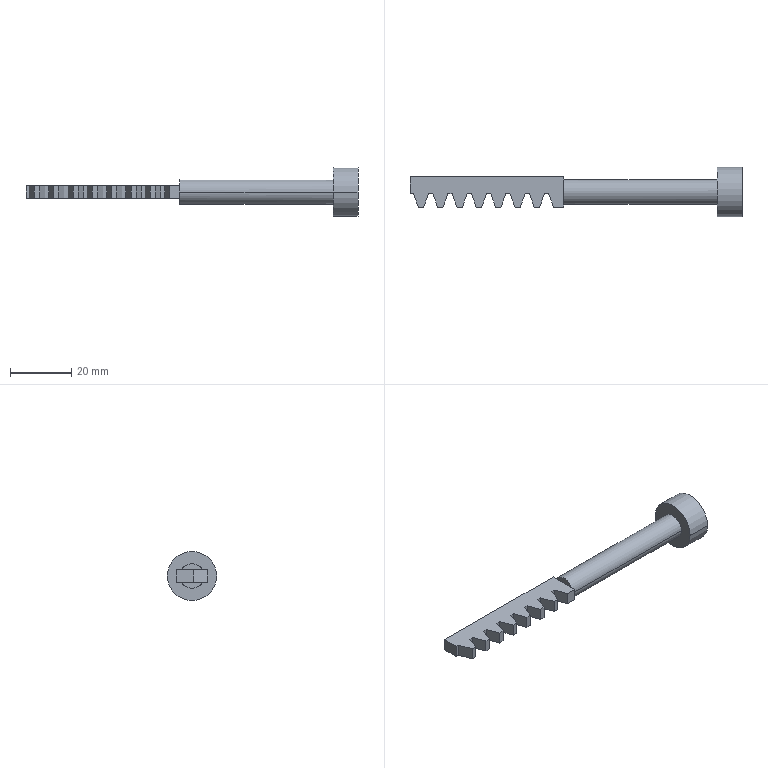Part | SolidWorks | features ICE 8, Extrusion 1, Revolution 1 | 1 solid | 45 faces | box 108 x 16 x 16 mm | volume 5714 mm3 | plane 41 | cylinder 4 | commonest cylinder face diameters 8 x2 16 x2
STEP:
#1=CARTESIAN_POINT('',(50.,13.,0.));
#2=VERTEX_POINT('',#1);
#3=CARTESIAN_POINT('',(50.,-3.,0.));
#4=VERTEX_POINT('',#3);
#5=CARTESIAN_POINT('',(50.,5.,0.));
#6=DIRECTION('',(1.,0.,0.));
#7=DIRECTION('',(0.,1.,0.));
#8=AXIS2_PLACEMENT_3D('',#5,#6,#7);
#9=CIRCLE('',#8,8.);
#10=EDGE_CURVE('',#2,#4,#9,.T.);
#11=ORIENTED_EDGE('',*,*,#10,.T.);
#12=CARTESIAN_POINT('',(58.,-3.,0.));
#13=VERTEX_POINT('',#12);
#14=CARTESIAN_POINT('',(0.,-3.,0.));
#15=DIRECTION('',(1.,0.,0.));
#16=VECTOR('',#15,1000.);
#17=LINE('',#14,#16);
#18=EDGE_CURVE('',#4,#13,#17,.T.);
#19=ORIENTED_EDGE('',*,*,#18,.T.);
#20=CARTESIAN_POINT('',(58.,13.,0.));
#21=VERTEX_POINT('',#20);
#22=CARTESIAN_POINT('',(58.,5.,0.));
#23=DIRECTION('',(1.,0.,0.));
#24=DIRECTION('',(0.,1.,0.));
#25=AXIS2_PLACEMENT_3D('',#22,#23,#24);
#26=CIRCLE('',#25,8.);
#27=EDGE_CURVE('',#21,#13,#26,.T.);
#28=ORIENTED_EDGE('',*,*,#27,.F.);
#29=CARTESIAN_POINT('',(0.,13.,0.));
#30=DIRECTION('',(1.,0.,0.));
#31=VECTOR('',#30,1000.);
#32=LINE('',#29,#31);
#33=EDGE_CURVE('',#2,#21,#32,.T.);
#34=ORIENTED_EDGE('',*,*,#33,.F.);
#35=EDGE_LOOP('',(#11,#19,#28,#34));
#36=FACE_OUTER_BOUND('',#35,.T.);
#37=CARTESIAN_POINT('',(0.,5.,0.));
#38=DIRECTION('',(1.,0.,0.));
#39=DIRECTION('',(0.,1.,0.));
#40=AXIS2_PLACEMENT_3D('',#37,#38,#39);
#41=CYLINDRICAL_SURFACE('',#40,8.);
#42=ADVANCED_FACE('',(#36),#41,.T.);
#43=CARTESIAN_POINT('',(0.,1.536,2.));
#44=VERTEX_POINT('',#43);
#45=CARTESIAN_POINT('',(0.,1.,0.));
#46=VERTEX_POINT('',#45);
#47=CARTESIAN_POINT('',(0.,5.,0.));
#48=DIRECTION('',(1.,0.,0.));
#49=DIRECTION('',(0.,1.,0.));
#50=AXIS2_PLACEMENT_3D('',#47,#48,#49);
#51=CIRCLE('',#50,4.);
#52=EDGE_CURVE('',#44,#46,#51,.T.);
#53=ORIENTED_EDGE('',*,*,#52,.T.);
#54=CARTESIAN_POINT('',(50.,1.,0.));
#55=VERTEX_POINT('',#54);
#56=CARTESIAN_POINT('',(0.,1.,0.));
#57=DIRECTION('',(1.,0.,0.));
#58=VECTOR('',#57,1000.);
#59=LINE('',#56,#58);
#60=EDGE_CURVE('',#46,#55,#59,.T.);
#61=ORIENTED_EDGE('',*,*,#60,.T.);
#62=CARTESIAN_POINT('',(50.,9.,0.));
#63=VERTEX_POINT('',#62);
#64=CARTESIAN_POINT('',(50.,5.,0.));
#65=DIRECTION('',(1.,0.,0.));
#66=DIRECTION('',(0.,1.,0.));
#67=AXIS2_PLACEMENT_3D('',#64,#65,#66);
#68=CIRCLE('',#67,4.);
#69=EDGE_CURVE('',#63,#55,#68,.T.);
#70=ORIENTED_EDGE('',*,*,#69,.F.);
#71=CARTESIAN_POINT('',(0.,9.,0.));
#72=VERTEX_POINT('',#71);
#73=CARTESIAN_POINT('',(0.,9.,0.));
#74=DIRECTION('',(1.,0.,0.));
#75=VECTOR('',#74,1000.);
#76=LINE('',#73,#75);
#77=EDGE_CURVE('',#72,#63,#76,.T.);
#78=ORIENTED_EDGE('',*,*,#77,.F.);
#79=CARTESIAN_POINT('',(0.,8.464,2.));
#80=VERTEX_POINT('',#79);
#81=CARTESIAN_POINT('',(0.,5.,0.));
#82=DIRECTION('',(1.,0.,0.));
#83=DIRECTION('',(0.,1.,0.));
#84=AXIS2_PLACEMENT_3D('',#81,#82,#83);
#85=CIRCLE('',#84,4.);
#86=EDGE_CURVE('',#72,#80,#85,.T.);
#87=ORIENTED_EDGE('',*,*,#86,.T.);
#88=CARTESIAN_POINT('',(0.,5.,0.));
#89=DIRECTION('',(1.,0.,0.));
#90=DIRECTION('',(0.,1.,0.));
#91=AXIS2_PLACEMENT_3D('',#88,#89,#90);
#92=CIRCLE('',#91,4.);
#93=EDGE_CURVE('',#80,#44,#92,.T.);
#94=ORIENTED_EDGE('',*,*,#93,.T.);
#95=EDGE_LOOP('',(#53,#61,#70,#78,#87,#94));
#96=FACE_OUTER_BOUND('',#95,.T.);
#97=CARTESIAN_POINT('',(0.,5.,0.));
#98=DIRECTION('',(1.,0.,0.));
#99=DIRECTION('',(0.,1.,0.));
#100=AXIS2_PLACEMENT_3D('',#97,#98,#99);
#101=CYLINDRICAL_SURFACE('',#100,4.);
#102=ADVANCED_FACE('',(#96),#101,.T.);
#103=ORIENTED_EDGE('',*,*,#52,.F.);
#104=CARTESIAN_POINT('',(0.,0.,2.));
#105=VERTEX_POINT('',#104);
#106=CARTESIAN_POINT('',(0.,0.,2.));
#107=DIRECTION('',(0.,1.,0.));
#108=VECTOR('',#107,1000.);
#109=LINE('',#106,#108);
#110=EDGE_CURVE('',#105,#44,#109,.T.);
#111=ORIENTED_EDGE('',*,*,#110,.F.);
#112=CARTESIAN_POINT('',(0.,0.,-2.));
#113=VERTEX_POINT('',#112);
#114=CARTESIAN_POINT('',(0.,0.,-2.));
#115=DIRECTION('',(0.,0.,1.));
#116=VECTOR('',#115,1000.);
#117=LINE('',#114,#116);
#118=EDGE_CURVE('',#113,#105,#117,.T.);
#119=ORIENTED_EDGE('',*,*,#118,.F.);
#120=CARTESIAN_POINT('',(0.,1.536,-2.));
#121=VERTEX_POINT('',#120);
#122=CARTESIAN_POINT('',(0.,0.,-2.));
#123=DIRECTION('',(0.,1.,0.));
#124=VECTOR('',#123,1000.);
#125=LINE('',#122,#124);
#126=EDGE_CURVE('',#113,#121,#125,.T.);
#127=ORIENTED_EDGE('',*,*,#126,.T.);
#128=CARTESIAN_POINT('',(0.,5.,0.));
#129=DIRECTION('',(1.,0.,0.));
#130=DIRECTION('',(0.,1.,0.));
#131=AXIS2_PLACEMENT_3D('',#128,#129,#130);
#132=CIRCLE('',#131,4.);
#133=EDGE_CURVE('',#46,#121,#132,.T.);
#134=ORIENTED_EDGE('',*,*,#133,.F.);
#135=EDGE_LOOP('',(#103,#111,#119,#127,#134));
#136=FACE_OUTER_BOUND('',#135,.T.);
#137=CARTESIAN_POINT('',(0.,0.,-2.));
#138=DIRECTION('',(1.,0.,0.));
#139=DIRECTION('',(0.,1.,0.));
#140=AXIS2_PLACEMENT_3D('',#137,#138,#139);
#141=PLANE('',#140);
#142=ADVANCED_FACE('',(#136),#141,.T.);
#143=CARTESIAN_POINT('',(-3.272,0.,2.));
#144=VERTEX_POINT('',#143);
#145=CARTESIAN_POINT('',(-3.272,0.,-2.));
#146=VERTEX_POINT('',#145);
#147=CARTESIAN_POINT('',(-3.272,0.,2.));
#148=DIRECTION('',(0.,0.,-1.));
#149=VECTOR('',#148,1000.);
#150=LINE('',#147,#149);
#151=EDGE_CURVE('',#144,#146,#150,.T.);
#152=ORIENTED_EDGE('',*,*,#151,.T.);
#153=CARTESIAN_POINT('',(-50.,0.,-2.));
#154=DIRECTION('',(1.,0.,0.));
#155=VECTOR('',#154,1000.);
#156=LINE('',#153,#155);
#157=EDGE_CURVE('',#146,#113,#156,.T.);
#158=ORIENTED_EDGE('',*,*,#157,.T.);
#159=ORIENTED_EDGE('',*,*,#118,.T.);
#160=CARTESIAN_POINT('',(-50.,0.,2.));
#161=DIRECTION('',(1.,0.,0.));
#162=VECTOR('',#161,1000.);
#163=LINE('',#160,#162);
#164=EDGE_CURVE('',#144,#105,#163,.T.);
#165=ORIENTED_EDGE('',*,*,#164,.F.);
#166=EDGE_LOOP('',(#152,#158,#159,#165));
#167=FACE_OUTER_BOUND('',#166,.T.);
#168=CARTESIAN_POINT('',(-50.,0.,-2.));
#169=DIRECTION('',(0.,-1.,0.));
#170=DIRECTION('',(0.,0.,-1.));
#171=AXIS2_PLACEMENT_3D('',#168,#169,#170);
#172=PLANE('',#171);
#173=ADVANCED_FACE('',(#167),#172,.T.);
#174=CARTESIAN_POINT('',(-7.87,0.,2.));
#175=VERTEX_POINT('',#174);
#176=CARTESIAN_POINT('',(-7.87,0.,-2.));
#177=VERTEX_POINT('',#176);
#178=CARTESIAN_POINT('',(-7.87,0.,2.));
#179=DIRECTION('',(0.,0.,-1.));
#180=VECTOR('',#179,1000.);
#181=LINE('',#178,#180);
#182=EDGE_CURVE('',#175,#177,#181,.T.);
#183=ORIENTED_EDGE('',*,*,#182,.F.);
#184=CARTESIAN_POINT('',(-9.556,0.,2.));
#185=VERTEX_POINT('',#184);
#186=CARTESIAN_POINT('',(-50.,0.,2.));
#187=DIRECTION('',(1.,0.,0.));
#188=VECTOR('',#187,1000.);
#189=LINE('',#186,#188);
#190=EDGE_CURVE('',#185,#175,#189,.T.);
#191=ORIENTED_EDGE('',*,*,#190,.F.);
#192=CARTESIAN_POINT('',(-9.556,0.,-2.));
#193=VERTEX_POINT('',#192);
#194=CARTESIAN_POINT('',(-9.556,0.,2.));
#195=DIRECTION('',(0.,0.,-1.));
#196=VECTOR('',#195,1000.);
#197=LINE('',#194,#196);
#198=EDGE_CURVE('',#185,#193,#197,.T.);
#199=ORIENTED_EDGE('',*,*,#198,.T.);
#200=CARTESIAN_POINT('',(-50.,0.,-2.));
#201=DIRECTION('',(1.,0.,0.));
#202=VECTOR('',#201,1000.);
#203=LINE('',#200,#202);
#204=EDGE_CURVE('',#193,#177,#203,.T.);
#205=ORIENTED_EDGE('',*,*,#204,.T.);
#206=EDGE_LOOP('',(#183,#191,#199,#205));
#207=FACE_OUTER_BOUND('',#206,.T.);
#208=CARTESIAN_POINT('',(-50.,0.,-2.));
#209=DIRECTION('',(0.,-1.,0.));
#210=DIRECTION('',(0.,0.,-1.));
#211=AXIS2_PLACEMENT_3D('',#208,#209,#210);
#212=PLANE('',#211);
#213=ADVANCED_FACE('',(#207),#212,.T.);
#214=CARTESIAN_POINT('',(-14.154,0.,2.));
#215=VERTEX_POINT('',#214);
#216=CARTESIAN_POINT('',(-14.154,0.,-2.));
#217=VERTEX_POINT('',#216);
#218=CARTESIAN_POINT('',(-14.154,0.,2.));
#219=DIRECTION('',(0.,0.,-1.));
#220=VECTOR('',#219,1000.);
#221=LINE('',#218,#220);
#222=EDGE_CURVE('',#215,#217,#221,.T.);
#223=ORIENTED_EDGE('',*,*,#222,.F.);
#224=CARTESIAN_POINT('',(-15.84,0.,2.));
#225=VERTEX_POINT('',#224);
#226=CARTESIAN_POINT('',(-50.,0.,2.));
#227=DIRECTION('',(1.,0.,0.));
#228=VECTOR('',#227,1000.);
#229=LINE('',#226,#228);
#230=EDGE_CURVE('',#225,#215,#229,.T.);
#231=ORIENTED_EDGE('',*,*,#230,.F.);
#232=CARTESIAN_POINT('',(-15.84,0.,-2.));
#233=VERTEX_POINT('',#232);
#234=CARTESIAN_POINT('',(-15.84,0.,2.));
#235=DIRECTION('',(0.,0.,-1.));
#236=VECTOR('',#235,1000.);
#237=LINE('',#234,#236);
#238=EDGE_CURVE('',#225,#233,#237,.T.);
#239=ORIENTED_EDGE('',*,*,#238,.T.);
#240=CARTESIAN_POINT('',(-50.,0.,-2.));
#241=DIRECTION('',(1.,0.,0.));
#242=VECTOR('',#241,1000.);
#243=LINE('',#240,#242);
#244=EDGE_CURVE('',#233,#217,#243,.T.);
#245=ORIENTED_EDGE('',*,*,#244,.T.);
#246=EDGE_LOOP('',(#223,#231,#239,#245));
#247=FACE_OUTER_BOUND('',#246,.T.);
#248=CARTESIAN_POINT('',(-50.,0.,-2.));
#249=DIRECTION('',(0.,-1.,0.));
#250=DIRECTION('',(0.,0.,-1.));
#251=AXIS2_PLACEMENT_3D('',#248,#249,#250);
#252=PLANE('',#251);
#253=ADVANCED_FACE('',(#247),#252,.T.);
#254=CARTESIAN_POINT('',(-20.438,0.,2.));
#255=VERTEX_POINT('',#254);
#256=CARTESIAN_POINT('',(-20.438,0.,-2.));
#257=VERTEX_POINT('',#256);
#258=CARTESIAN_POINT('',(-20.438,0.,2.));
#259=DIRECTION('',(0.,0.,-1.));
#260=VECTOR('',#259,1000.);
#261=LINE('',#258,#260);
#262=EDGE_CURVE('',#255,#257,#261,.T.);
#263=ORIENTED_EDGE('',*,*,#262,.F.);
#264=CARTESIAN_POINT('',(-22.124,0.,2.));
#265=VERTEX_POINT('',#264);
#266=CARTESIAN_POINT('',(-50.,0.,2.));
#267=DIRECTION('',(1.,0.,0.));
#268=VECTOR('',#267,1000.);
#269=LINE('',#266,#268);
#270=EDGE_CURVE('',#265,#255,#269,.T.);
#271=ORIENTED_EDGE('',*,*,#270,.F.);
#272=CARTESIAN_POINT('',(-22.124,0.,-2.));
#273=VERTEX_POINT('',#272);
#274=CARTESIAN_POINT('',(-22.124,0.,2.));
#275=DIRECTION('',(0.,0.,-1.));
#276=VECTOR('',#275,1000.);
#277=LINE('',#274,#276);
#278=EDGE_CURVE('',#265,#273,#277,.T.);
#279=ORIENTED_EDGE('',*,*,#278,.T.);
#280=CARTESIAN_POINT('',(-50.,0.,-2.));
#281=DIRECTION('',(1.,0.,0.));
#282=VECTOR('',#281,1000.);
#283=LINE('',#280,#282);
#284=EDGE_CURVE('',#273,#257,#283,.T.);
#285=ORIENTED_EDGE('',*,*,#284,.T.);
#286=EDGE_LOOP('',(#263,#271,#279,#285));
#287=FACE_OUTER_BOUND('',#286,.T.);
#288=CARTESIAN_POINT('',(-50.,0.,-2.));
#289=DIRECTION('',(0.,-1.,0.));
#290=DIRECTION('',(0.,0.,-1.));
#291=AXIS2_PLACEMENT_3D('',#288,#289,#290);
#292=PLANE('',#291);
#293=ADVANCED_FACE('',(#287),#292,.T.);
#294=CARTESIAN_POINT('',(-26.722,0.,2.));
#295=VERTEX_POINT('',#294);
#296=CARTESIAN_POINT('',(-26.722,0.,-2.));
#297=VERTEX_POINT('',#296);
#298=CARTESIAN_POINT('',(-26.722,0.,2.));
#299=DIRECTION('',(0.,0.,-1.));
#300=VECTOR('',#299,1000.);
#301=LINE('',#298,#300);
#302=EDGE_CURVE('',#295,#297,#301,.T.);
#303=ORIENTED_EDGE('',*,*,#302,.F.);
#304=CARTESIAN_POINT('',(-28.408,0.,2.));
#305=VERTEX_POINT('',#304);
#306=CARTESIAN_POINT('',(-50.,0.,2.));
#307=DIRECTION('',(1.,0.,0.));
#308=VECTOR('',#307,1000.);
#309=LINE('',#306,#308);
#310=EDGE_CURVE('',#305,#295,#309,.T.);
#311=ORIENTED_EDGE('',*,*,#310,.F.);
#312=CARTESIAN_POINT('',(-28.408,0.,-2.));
#313=VERTEX_POINT('',#312);
#314=CARTESIAN_POINT('',(-28.408,0.,2.));
#315=DIRECTION('',(0.,0.,-1.));
#316=VECTOR('',#315,1000.);
#317=LINE('',#314,#316);
#318=EDGE_CURVE('',#305,#313,#317,.T.);
#319=ORIENTED_EDGE('',*,*,#318,.T.);
#320=CARTESIAN_POINT('',(-50.,0.,-2.));
#321=DIRECTION('',(1.,0.,0.));
#322=VECTOR('',#321,1000.);
#323=LINE('',#320,#322);
#324=EDGE_CURVE('',#313,#297,#323,.T.);
#325=ORIENTED_EDGE('',*,*,#324,.T.);
#326=EDGE_LOOP('',(#303,#311,#319,#325));
#327=FACE_OUTER_BOUND('',#326,.T.);
#328=CARTESIAN_POINT('',(-50.,0.,-2.));
#329=DIRECTION('',(0.,-1.,0.));
#330=DIRECTION('',(0.,0.,-1.));
#331=AXIS2_PLACEMENT_3D('',#328,#329,#330);
#332=PLANE('',#331);
#333=ADVANCED_FACE('',(#327),#332,.T.);
#334=CARTESIAN_POINT('',(-33.006,0.,2.));
#335=VERTEX_POINT('',#334);
#336=CARTESIAN_POINT('',(-33.006,0.,-2.));
#337=VERTEX_POINT('',#336);
#338=CARTESIAN_POINT('',(-33.006,0.,2.));
#339=DIRECTION('',(0.,0.,-1.));
#340=VECTOR('',#339,1000.);
#341=LINE('',#338,#340);
#342=EDGE_CURVE('',#335,#337,#341,.T.);
#343=ORIENTED_EDGE('',*,*,#342,.F.);
#344=CARTESIAN_POINT('',(-34.692,0.,2.));
#345=VERTEX_POINT('',#344);
#346=CARTESIAN_POINT('',(-50.,0.,2.));
#347=DIRECTION('',(1.,0.,0.));
#348=VECTOR('',#347,1000.);
#349=LINE('',#346,#348);
#350=EDGE_CURVE('',#345,#335,#349,.T.);
#351=ORIENTED_EDGE('',*,*,#350,.F.);
#352=CARTESIAN_POINT('',(-34.692,0.,-2.));
#353=VERTEX_POINT('',#352);
#354=CARTESIAN_POINT('',(-34.692,0.,2.));
#355=DIRECTION('',(0.,0.,-1.));
#356=VECTOR('',#355,1000.);
#357=LINE('',#354,#356);
#358=EDGE_CURVE('',#345,#353,#357,.T.);
#359=ORIENTED_EDGE('',*,*,#358,.T.);
#360=CARTESIAN_POINT('',(-50.,0.,-2.));
#361=DIRECTION('',(1.,0.,0.));
#362=VECTOR('',#361,1000.);
#363=LINE('',#360,#362);
#364=EDGE_CURVE('',#353,#337,#363,.T.);
#365=ORIENTED_EDGE('',*,*,#364,.T.);
#366=EDGE_LOOP('',(#343,#351,#359,#365));
#367=FACE_OUTER_BOUND('',#366,.T.);
#368=CARTESIAN_POINT('',(-50.,0.,-2.));
#369=DIRECTION('',(0.,-1.,0.));
#370=DIRECTION('',(0.,0.,-1.));
#371=AXIS2_PLACEMENT_3D('',#368,#369,#370);
#372=PLANE('',#371);
#373=ADVANCED_FACE('',(#367),#372,.T.);
#374=CARTESIAN_POINT('',(-39.29,0.,2.));
#375=VERTEX_POINT('',#374);
#376=CARTESIAN_POINT('',(-39.29,0.,-2.));
#377=VERTEX_POINT('',#376);
#378=CARTESIAN_POINT('',(-39.29,0.,2.));
#379=DIRECTION('',(0.,0.,-1.));
#380=VECTOR('',#379,1000.);
#381=LINE('',#378,#380);
#382=EDGE_CURVE('',#375,#377,#381,.T.);
#383=ORIENTED_EDGE('',*,*,#382,.F.);
#384=CARTESIAN_POINT('',(-40.976,0.,2.));
#385=VERTEX_POINT('',#384);
#386=CARTESIAN_POINT('',(-50.,0.,2.));
#387=DIRECTION('',(1.,0.,0.));
#388=VECTOR('',#387,1000.);
#389=LINE('',#386,#388);
#390=EDGE_CURVE('',#385,#375,#389,.T.);
#391=ORIENTED_EDGE('',*,*,#390,.F.);
#392=CARTESIAN_POINT('',(-40.976,0.,-2.));
#393=VERTEX_POINT('',#392);
#394=CARTESIAN_POINT('',(-40.976,0.,2.));
#395=DIRECTION('',(0.,0.,-1.));
#396=VECTOR('',#395,1000.);
#397=LINE('',#394,#396);
#398=EDGE_CURVE('',#385,#393,#397,.T.);
#399=ORIENTED_EDGE('',*,*,#398,.T.);
#400=CARTESIAN_POINT('',(-50.,0.,-2.));
#401=DIRECTION('',(1.,0.,0.));
#402=VECTOR('',#401,1000.);
#403=LINE('',#400,#402);
#404=EDGE_CURVE('',#393,#377,#403,.T.);
#405=ORIENTED_EDGE('',*,*,#404,.T.);
#406=EDGE_LOOP('',(#383,#391,#399,#405));
#407=FACE_OUTER_BOUND('',#406,.T.);
#408=CARTESIAN_POINT('',(-50.,0.,-2.));
#409=DIRECTION('',(0.,-1.,0.));
#410=DIRECTION('',(0.,0.,-1.));
#411=AXIS2_PLACEMENT_3D('',#408,#409,#410);
#412=PLANE('',#411);
#413=ADVANCED_FACE('',(#407),#412,.T.);
#414=CARTESIAN_POINT('',(0.,10.,2.));
#415=VERTEX_POINT('',#414);
#416=CARTESIAN_POINT('',(-50.,10.,2.));
#417=VERTEX_POINT('',#416);
#418=CARTESIAN_POINT('',(0.,10.,2.));
#419=DIRECTION('',(-1.,0.,0.));
#420=VECTOR('',#419,1000.);
#421=LINE('',#418,#420);
#422=EDGE_CURVE('',#415,#417,#421,.T.);
#423=ORIENTED_EDGE('',*,*,#422,.F.);
#424=CARTESIAN_POINT('',(0.,10.,-2.));
#425=VERTEX_POINT('',#424);
#426=CARTESIAN_POINT('',(0.,10.,-2.));
#427=DIRECTION('',(0.,0.,1.));
#428=VECTOR('',#427,1000.);
#429=LINE('',#426,#428);
#430=EDGE_CURVE('',#425,#415,#429,.T.);
#431=ORIENTED_EDGE('',*,*,#430,.F.);
#432=CARTESIAN_POINT('',(-50.,10.,-2.));
#433=VERTEX_POINT('',#432);
#434=CARTESIAN_POINT('',(0.,10.,-2.));
#435=DIRECTION('',(-1.,0.,0.));
#436=VECTOR('',#435,1000.);
#437=LINE('',#434,#436);
#438=EDGE_CURVE('',#425,#433,#437,.T.);
#439=ORIENTED_EDGE('',*,*,#438,.T.);
#440=CARTESIAN_POINT('',(-50.,10.,-2.));
#441=DIRECTION('',(0.,0.,1.));
#442=VECTOR('',#441,1000.);
#443=LINE('',#440,#442);
#444=EDGE_CURVE('',#433,#417,#443,.T.);
#445=ORIENTED_EDGE('',*,*,#444,.T.);
#446=EDGE_LOOP('',(#423,#431,#439,#445));
#447=FACE_OUTER_BOUND('',#446,.T.);
#448=CARTESIAN_POINT('',(0.,10.,-2.));
#449=DIRECTION('',(0.,1.,0.));
#450=DIRECTION('',(0.,0.,1.));
#451=AXIS2_PLACEMENT_3D('',#448,#449,#450);
#452=PLANE('',#451);
#453=ADVANCED_FACE('',(#447),#452,.T.);
#454=CARTESIAN_POINT('',(0.,8.464,-2.));
#455=VERTEX_POINT('',#454);
#456=CARTESIAN_POINT('',(0.,5.,0.));
#457=DIRECTION('',(1.,0.,0.));
#458=DIRECTION('',(0.,1.,0.));
#459=AXIS2_PLACEMENT_3D('',#456,#457,#458);
#460=CIRCLE('',#459,4.);
#461=EDGE_CURVE('',#455,#72,#460,.T.);
#462=ORIENTED_EDGE('',*,*,#461,.F.);
#463=CARTESIAN_POINT('',(0.,0.,-2.));
#464=DIRECTION('',(0.,1.,0.));
#465=VECTOR('',#464,1000.);
#466=LINE('',#463,#465);
#467=EDGE_CURVE('',#455,#425,#466,.T.);
#468=ORIENTED_EDGE('',*,*,#467,.T.);
#469=ORIENTED_EDGE('',*,*,#430,.T.);
#470=CARTESIAN_POINT('',(0.,0.,2.));
#471=DIRECTION('',(0.,1.,0.));
#472=VECTOR('',#471,1000.);
#473=LINE('',#470,#472);
#474=EDGE_CURVE('',#80,#415,#473,.T.);
#475=ORIENTED_EDGE('',*,*,#474,.F.);
#476=ORIENTED_EDGE('',*,*,#86,.F.);
#477=EDGE_LOOP('',(#462,#468,#469,#475,#476));
#478=FACE_OUTER_BOUND('',#477,.T.);
#479=CARTESIAN_POINT('',(0.,0.,-2.));
#480=DIRECTION('',(1.,0.,0.));
#481=DIRECTION('',(0.,1.,0.));
#482=AXIS2_PLACEMENT_3D('',#479,#480,#481);
#483=PLANE('',#482);
#484=ADVANCED_FACE('',(#478),#483,.T.);
#485=CARTESIAN_POINT('',(-47.26,0.,2.));
#486=VERTEX_POINT('',#485);
#487=CARTESIAN_POINT('',(-47.26,0.,-2.));
#488=VERTEX_POINT('',#487);
#489=CARTESIAN_POINT('',(-47.26,0.,2.));
#490=DIRECTION('',(0.,0.,-1.));
#491=VECTOR('',#490,1000.);
#492=LINE('',#489,#491);
#493=EDGE_CURVE('',#486,#488,#492,.T.);
#494=ORIENTED_EDGE('',*,*,#493,.T.);
#495=CARTESIAN_POINT('',(-45.574,0.,-2.));
#496=VERTEX_POINT('',#495);
#497=CARTESIAN_POINT('',(-50.,0.,-2.));
#498=DIRECTION('',(1.,0.,0.));
#499=VECTOR('',#498,1000.);
#500=LINE('',#497,#499);
#501=EDGE_CURVE('',#488,#496,#500,.T.);
#502=ORIENTED_EDGE('',*,*,#501,.T.);
#503=CARTESIAN_POINT('',(-45.574,0.,2.));
#504=VERTEX_POINT('',#503);
#505=CARTESIAN_POINT('',(-45.574,0.,2.));
#506=DIRECTION('',(0.,0.,-1.));
#507=VECTOR('',#506,1000.);
#508=LINE('',#505,#507);
#509=EDGE_CURVE('',#504,#496,#508,.T.);
#510=ORIENTED_EDGE('',*,*,#509,.F.);
#511=CARTESIAN_POINT('',(-50.,0.,2.));
#512=DIRECTION('',(1.,0.,0.));
#513=VECTOR('',#512,1000.);
#514=LINE('',#511,#513);
#515=EDGE_CURVE('',#486,#504,#514,.T.);
#516=ORIENTED_EDGE('',*,*,#515,.F.);
#517=EDGE_LOOP('',(#494,#502,#510,#516));
#518=FACE_OUTER_BOUND('',#517,.T.);
#519=CARTESIAN_POINT('',(-50.,0.,-2.));
#520=DIRECTION('',(0.,-1.,0.));
#521=DIRECTION('',(0.,0.,-1.));
#522=AXIS2_PLACEMENT_3D('',#519,#520,#521);
#523=PLANE('',#522);
#524=ADVANCED_FACE('',(#518),#523,.T.);
#525=CARTESIAN_POINT('',(-50.,4.5,2.));
#526=VERTEX_POINT('',#525);
#527=CARTESIAN_POINT('',(-50.,4.5,-2.));
#528=VERTEX_POINT('',#527);
#529=CARTESIAN_POINT('',(-50.,4.5,2.));
#530=DIRECTION('',(0.,0.,-1.));
#531=VECTOR('',#530,1000.);
#532=LINE('',#529,#531);
#533=EDGE_CURVE('',#526,#528,#532,.T.);
#534=ORIENTED_EDGE('',*,*,#533,.F.);
#535=CARTESIAN_POINT('',(-50.,10.,2.));
#536=DIRECTION('',(0.,-1.,0.));
#537=VECTOR('',#536,1000.);
#538=LINE('',#535,#537);
#539=EDGE_CURVE('',#417,#526,#538,.T.);
#540=ORIENTED_EDGE('',*,*,#539,.F.);
#541=ORIENTED_EDGE('',*,*,#444,.F.);
#542=CARTESIAN_POINT('',(-50.,10.,-2.));
#543=DIRECTION('',(0.,-1.,0.));
#544=VECTOR('',#543,1000.);
#545=LINE('',#542,#544);
#546=EDGE_CURVE('',#433,#528,#545,.T.);
#547=ORIENTED_EDGE('',*,*,#546,.T.);
#548=EDGE_LOOP('',(#534,#540,#541,#547));
#549=FACE_OUTER_BOUND('',#548,.T.);
#550=CARTESIAN_POINT('',(-50.,10.,-2.));
#551=DIRECTION('',(-1.,0.,0.));
#552=DIRECTION('',(0.,0.,1.));
#553=AXIS2_PLACEMENT_3D('',#550,#551,#552);
#554=PLANE('',#553);
#555=ADVANCED_FACE('',(#549),#554,.T.);
#556=CARTESIAN_POINT('',(-48.898,4.5,-2.));
#557=VERTEX_POINT('',#556);
#558=CARTESIAN_POINT('',(-48.898,4.5,-2.));
#559=DIRECTION('',(0.342,-0.9397,0.));
#560=VECTOR('',#559,1000.);
#561=LINE('',#558,#560);
#562=EDGE_CURVE('',#557,#488,#561,.T.);
#563=ORIENTED_EDGE('',*,*,#562,.F.);
#564=CARTESIAN_POINT('',(-50.,4.5,-2.));
#565=DIRECTION('',(1.,0.,0.));
#566=VECTOR('',#565,1000.);
#567=LINE('',#564,#566);
#568=EDGE_CURVE('',#528,#557,#567,.T.);
#569=ORIENTED_EDGE('',*,*,#568,.F.);
#570=ORIENTED_EDGE('',*,*,#546,.F.);
#571=ORIENTED_EDGE('',*,*,#438,.F.);
#572=ORIENTED_EDGE('',*,*,#467,.F.);
#573=CARTESIAN_POINT('',(0.,0.,-2.));
#574=DIRECTION('',(0.,1.,0.));
#575=VECTOR('',#574,1000.);
#576=LINE('',#573,#575);
#577=EDGE_CURVE('',#121,#455,#576,.T.);
#578=ORIENTED_EDGE('',*,*,#577,.F.);
#579=ORIENTED_EDGE('',*,*,#126,.F.);
#580=ORIENTED_EDGE('',*,*,#157,.F.);
#581=CARTESIAN_POINT('',(-4.91,4.5,-2.));
#582=VERTEX_POINT('',#581);
#583=CARTESIAN_POINT('',(-4.91,4.5,-2.));
#584=DIRECTION('',(0.342,-0.9397,0.));
#585=VECTOR('',#584,1000.);
#586=LINE('',#583,#585);
#587=EDGE_CURVE('',#582,#146,#586,.T.);
#588=ORIENTED_EDGE('',*,*,#587,.F.);
#589=CARTESIAN_POINT('',(-6.232,4.5,-2.));
#590=VERTEX_POINT('',#589);
#591=CARTESIAN_POINT('',(-6.232,4.5,-2.));
#592=DIRECTION('',(1.,0.,0.));
#593=VECTOR('',#592,1000.);
#594=LINE('',#591,#593);
#595=EDGE_CURVE('',#590,#582,#594,.T.);
#596=ORIENTED_EDGE('',*,*,#595,.F.);
#597=CARTESIAN_POINT('',(-7.87,0.,-2.));
#598=DIRECTION('',(0.342,0.9397,0.));
#599=VECTOR('',#598,1000.);
#600=LINE('',#597,#599);
#601=EDGE_CURVE('',#177,#590,#600,.T.);
#602=ORIENTED_EDGE('',*,*,#601,.F.);
#603=ORIENTED_EDGE('',*,*,#204,.F.);
#604=CARTESIAN_POINT('',(-11.194,4.5,-2.));
#605=VERTEX_POINT('',#604);
#606=CARTESIAN_POINT('',(-11.194,4.5,-2.));
#607=DIRECTION('',(0.342,-0.9397,0.));
#608=VECTOR('',#607,1000.);
#609=LINE('',#606,#608);
#610=EDGE_CURVE('',#605,#193,#609,.T.);
#611=ORIENTED_EDGE('',*,*,#610,.F.);
#612=CARTESIAN_POINT('',(-12.516,4.5,-2.));
#613=VERTEX_POINT('',#612);
#614=CARTESIAN_POINT('',(-12.516,4.5,-2.));
#615=DIRECTION('',(1.,0.,0.));
#616=VECTOR('',#615,1000.);
#617=LINE('',#614,#616);
#618=EDGE_CURVE('',#613,#605,#617,.T.);
#619=ORIENTED_EDGE('',*,*,#618,.F.);
#620=CARTESIAN_POINT('',(-14.154,0.,-2.));
#621=DIRECTION('',(0.342,0.9397,0.));
#622=VECTOR('',#621,1000.);
#623=LINE('',#620,#622);
#624=EDGE_CURVE('',#217,#613,#623,.T.);
#625=ORIENTED_EDGE('',*,*,#624,.F.);
#626=ORIENTED_EDGE('',*,*,#244,.F.);
#627=CARTESIAN_POINT('',(-17.478,4.5,-2.));
#628=VERTEX_POINT('',#627);
#629=CARTESIAN_POINT('',(-17.478,4.5,-2.));
#630=DIRECTION('',(0.342,-0.9397,0.));
#631=VECTOR('',#630,1000.);
#632=LINE('',#629,#631);
#633=EDGE_CURVE('',#628,#233,#632,.T.);
#634=ORIENTED_EDGE('',*,*,#633,.F.);
#635=CARTESIAN_POINT('',(-18.8,4.5,-2.));
#636=VERTEX_POINT('',#635);
#637=CARTESIAN_POINT('',(-18.8,4.5,-2.));
#638=DIRECTION('',(1.,0.,0.));
#639=VECTOR('',#638,1000.);
#640=LINE('',#637,#639);
#641=EDGE_CURVE('',#636,#628,#640,.T.);
#642=ORIENTED_EDGE('',*,*,#641,.F.);
#643=CARTESIAN_POINT('',(-20.438,0.,-2.));
#644=DIRECTION('',(0.342,0.9397,0.));
#645=VECTOR('',#644,1000.);
#646=LINE('',#643,#645);
#647=EDGE_CURVE('',#257,#636,#646,.T.);
#648=ORIENTED_EDGE('',*,*,#647,.F.);
#649=ORIENTED_EDGE('',*,*,#284,.F.);
#650=CARTESIAN_POINT('',(-23.762,4.5,-2.));
#651=VERTEX_POINT('',#650);
#652=CARTESIAN_POINT('',(-23.762,4.5,-2.));
#653=DIRECTION('',(0.342,-0.9397,0.));
#654=VECTOR('',#653,1000.);
#655=LINE('',#652,#654);
#656=EDGE_CURVE('',#651,#273,#655,.T.);
#657=ORIENTED_EDGE('',*,*,#656,.F.);
#658=CARTESIAN_POINT('',(-25.084,4.5,-2.));
#659=VERTEX_POINT('',#658);
#660=CARTESIAN_POINT('',(-25.084,4.5,-2.));
#661=DIRECTION('',(1.,0.,0.));
#662=VECTOR('',#661,1000.);
#663=LINE('',#660,#662);
#664=EDGE_CURVE('',#659,#651,#663,.T.);
#665=ORIENTED_EDGE('',*,*,#664,.F.);
#666=CARTESIAN_POINT('',(-26.722,0.,-2.));
#667=DIRECTION('',(0.342,0.9397,0.));
#668=VECTOR('',#667,1000.);
#669=LINE('',#666,#668);
#670=EDGE_CURVE('',#297,#659,#669,.T.);
#671=ORIENTED_EDGE('',*,*,#670,.F.);
#672=ORIENTED_EDGE('',*,*,#324,.F.);
#673=CARTESIAN_POINT('',(-30.046,4.5,-2.));
#674=VERTEX_POINT('',#673);
#675=CARTESIAN_POINT('',(-30.046,4.5,-2.));
#676=DIRECTION('',(0.342,-0.9397,0.));
#677=VECTOR('',#676,1000.);
#678=LINE('',#675,#677);
#679=EDGE_CURVE('',#674,#313,#678,.T.);
#680=ORIENTED_EDGE('',*,*,#679,.F.);
#681=CARTESIAN_POINT('',(-31.368,4.5,-2.));
#682=VERTEX_POINT('',#681);
#683=CARTESIAN_POINT('',(-31.368,4.5,-2.));
#684=DIRECTION('',(1.,0.,0.));
#685=VECTOR('',#684,1000.);
#686=LINE('',#683,#685);
#687=EDGE_CURVE('',#682,#674,#686,.T.);
#688=ORIENTED_EDGE('',*,*,#687,.F.);
#689=CARTESIAN_POINT('',(-33.006,0.,-2.));
#690=DIRECTION('',(0.342,0.9397,0.));
#691=VECTOR('',#690,1000.);
#692=LINE('',#689,#691);
#693=EDGE_CURVE('',#337,#682,#692,.T.);
#694=ORIENTED_EDGE('',*,*,#693,.F.);
#695=ORIENTED_EDGE('',*,*,#364,.F.);
#696=CARTESIAN_POINT('',(-36.33,4.5,-2.));
#697=VERTEX_POINT('',#696);
#698=CARTESIAN_POINT('',(-36.33,4.5,-2.));
#699=DIRECTION('',(0.342,-0.9397,0.));
#700=VECTOR('',#699,1000.);
#701=LINE('',#698,#700);
#702=EDGE_CURVE('',#697,#353,#701,.T.);
#703=ORIENTED_EDGE('',*,*,#702,.F.);
#704=CARTESIAN_POINT('',(-37.652,4.5,-2.));
#705=VERTEX_POINT('',#704);
#706=CARTESIAN_POINT('',(-37.652,4.5,-2.));
#707=DIRECTION('',(1.,0.,0.));
#708=VECTOR('',#707,1000.);
#709=LINE('',#706,#708);
#710=EDGE_CURVE('',#705,#697,#709,.T.);
#711=ORIENTED_EDGE('',*,*,#710,.F.);
#712=CARTESIAN_POINT('',(-39.29,0.,-2.));
#713=DIRECTION('',(0.342,0.9397,0.));
#714=VECTOR('',#713,1000.);
#715=LINE('',#712,#714);
#716=EDGE_CURVE('',#377,#705,#715,.T.);
#717=ORIENTED_EDGE('',*,*,#716,.F.);
#718=ORIENTED_EDGE('',*,*,#404,.F.);
#719=CARTESIAN_POINT('',(-42.614,4.5,-2.));
#720=VERTEX_POINT('',#719);
#721=CARTESIAN_POINT('',(-42.614,4.5,-2.));
#722=DIRECTION('',(0.342,-0.9397,0.));
#723=VECTOR('',#722,1000.);
#724=LINE('',#721,#723);
#725=EDGE_CURVE('',#720,#393,#724,.T.);
#726=ORIENTED_EDGE('',*,*,#725,.F.);
#727=CARTESIAN_POINT('',(-43.936,4.5,-2.));
#728=VERTEX_POINT('',#727);
#729=CARTESIAN_POINT('',(-43.936,4.5,-2.));
#730=DIRECTION('',(1.,0.,0.));
#731=VECTOR('',#730,1000.);
#732=LINE('',#729,#731);
#733=EDGE_CURVE('',#728,#720,#732,.T.);
#734=ORIENTED_EDGE('',*,*,#733,.F.);
#735=CARTESIAN_POINT('',(-45.574,0.,-2.));
#736=DIRECTION('',(0.342,0.9397,0.));
#737=VECTOR('',#736,1000.);
#738=LINE('',#735,#737);
#739=EDGE_CURVE('',#496,#728,#738,.T.);
#740=ORIENTED_EDGE('',*,*,#739,.F.);
#741=ORIENTED_EDGE('',*,*,#501,.F.);
#742=EDGE_LOOP('',(#563,#569,#570,#571,#572,#578,#579,#580,#588,#596,#602,#603,#611,#619,#625,#626,#634,#642,#648,#649,#657,#665,#671,#672,#680,#688,#694,#695,#703,#711,#717,#718,#726,#734,#740,#741));
#743=FACE_OUTER_BOUND('',#742,.T.);
#744=CARTESIAN_POINT('',(0.,0.,-2.));
#745=DIRECTION('',(0.,0.,1.));
#746=DIRECTION('',(1.,0.,0.));
#747=AXIS2_PLACEMENT_3D('',#744,#745,#746);
#748=PLANE('',#747);
#749=ADVANCED_FACE('',(#743),#748,.F.);
#750=CARTESIAN_POINT('',(-48.898,4.5,2.));
#751=VERTEX_POINT('',#750);
#752=CARTESIAN_POINT('',(-50.,4.5,2.));
#753=DIRECTION('',(1.,0.,0.));
#754=VECTOR('',#753,1000.);
#755=LINE('',#752,#754);
#756=EDGE_CURVE('',#526,#751,#755,.T.);
#757=ORIENTED_EDGE('',*,*,#756,.T.);
#758=CARTESIAN_POINT('',(-48.898,4.5,2.));
#759=DIRECTION('',(0.342,-0.9397,0.));
#760=VECTOR('',#759,1000.);
#761=LINE('',#758,#760);
#762=EDGE_CURVE('',#751,#486,#761,.T.);
#763=ORIENTED_EDGE('',*,*,#762,.T.);
#764=ORIENTED_EDGE('',*,*,#515,.T.);
#765=CARTESIAN_POINT('',(-43.936,4.5,2.));
#766=VERTEX_POINT('',#765);
#767=CARTESIAN_POINT('',(-45.574,0.,2.));
#768=DIRECTION('',(0.342,0.9397,0.));
#769=VECTOR('',#768,1000.);
#770=LINE('',#767,#769);
#771=EDGE_CURVE('',#504,#766,#770,.T.);
#772=ORIENTED_EDGE('',*,*,#771,.T.);
#773=CARTESIAN_POINT('',(-42.614,4.5,2.));
#774=VERTEX_POINT('',#773);
#775=CARTESIAN_POINT('',(-43.936,4.5,2.));
#776=DIRECTION('',(1.,0.,0.));
#777=VECTOR('',#776,1000.);
#778=LINE('',#775,#777);
#779=EDGE_CURVE('',#766,#774,#778,.T.);
#780=ORIENTED_EDGE('',*,*,#779,.T.);
#781=CARTESIAN_POINT('',(-42.614,4.5,2.));
#782=DIRECTION('',(0.342,-0.9397,0.));
#783=VECTOR('',#782,1000.);
#784=LINE('',#781,#783);
#785=EDGE_CURVE('',#774,#385,#784,.T.);
#786=ORIENTED_EDGE('',*,*,#785,.T.);
#787=ORIENTED_EDGE('',*,*,#390,.T.);
#788=CARTESIAN_POINT('',(-37.652,4.5,2.));
#789=VERTEX_POINT('',#788);
#790=CARTESIAN_POINT('',(-39.29,0.,2.));
#791=DIRECTION('',(0.342,0.9397,0.));
#792=VECTOR('',#791,1000.);
#793=LINE('',#790,#792);
#794=EDGE_CURVE('',#375,#789,#793,.T.);
#795=ORIENTED_EDGE('',*,*,#794,.T.);
#796=CARTESIAN_POINT('',(-36.33,4.5,2.));
#797=VERTEX_POINT('',#796);
#798=CARTESIAN_POINT('',(-37.652,4.5,2.));
#799=DIRECTION('',(1.,0.,0.));
#800=VECTOR('',#799,1000.);
#801=LINE('',#798,#800);
#802=EDGE_CURVE('',#789,#797,#801,.T.);
#803=ORIENTED_EDGE('',*,*,#802,.T.);
#804=CARTESIAN_POINT('',(-36.33,4.5,2.));
#805=DIRECTION('',(0.342,-0.9397,0.));
#806=VECTOR('',#805,1000.);
#807=LINE('',#804,#806);
#808=EDGE_CURVE('',#797,#345,#807,.T.);
#809=ORIENTED_EDGE('',*,*,#808,.T.);
#810=ORIENTED_EDGE('',*,*,#350,.T.);
#811=CARTESIAN_POINT('',(-31.368,4.5,2.));
#812=VERTEX_POINT('',#811);
#813=CARTESIAN_POINT('',(-33.006,0.,2.));
#814=DIRECTION('',(0.342,0.9397,0.));
#815=VECTOR('',#814,1000.);
#816=LINE('',#813,#815);
#817=EDGE_CURVE('',#335,#812,#816,.T.);
#818=ORIENTED_EDGE('',*,*,#817,.T.);
#819=CARTESIAN_POINT('',(-30.046,4.5,2.));
#820=VERTEX_POINT('',#819);
#821=CARTESIAN_POINT('',(-31.368,4.5,2.));
#822=DIRECTION('',(1.,0.,0.));
#823=VECTOR('',#822,1000.);
#824=LINE('',#821,#823);
#825=EDGE_CURVE('',#812,#820,#824,.T.);
#826=ORIENTED_EDGE('',*,*,#825,.T.);
#827=CARTESIAN_POINT('',(-30.046,4.5,2.));
#828=DIRECTION('',(0.342,-0.9397,0.));
#829=VECTOR('',#828,1000.);
#830=LINE('',#827,#829);
#831=EDGE_CURVE('',#820,#305,#830,.T.);
#832=ORIENTED_EDGE('',*,*,#831,.T.);
#833=ORIENTED_EDGE('',*,*,#310,.T.);
#834=CARTESIAN_POINT('',(-25.084,4.5,2.));
#835=VERTEX_POINT('',#834);
#836=CARTESIAN_POINT('',(-26.722,0.,2.));
#837=DIRECTION('',(0.342,0.9397,0.));
#838=VECTOR('',#837,1000.);
#839=LINE('',#836,#838);
#840=EDGE_CURVE('',#295,#835,#839,.T.);
#841=ORIENTED_EDGE('',*,*,#840,.T.);
#842=CARTESIAN_POINT('',(-23.762,4.5,2.));
#843=VERTEX_POINT('',#842);
#844=CARTESIAN_POINT('',(-25.084,4.5,2.));
#845=DIRECTION('',(1.,0.,0.));
#846=VECTOR('',#845,1000.);
#847=LINE('',#844,#846);
#848=EDGE_CURVE('',#835,#843,#847,.T.);
#849=ORIENTED_EDGE('',*,*,#848,.T.);
#850=CARTESIAN_POINT('',(-23.762,4.5,2.));
#851=DIRECTION('',(0.342,-0.9397,0.));
#852=VECTOR('',#851,1000.);
#853=LINE('',#850,#852);
#854=EDGE_CURVE('',#843,#265,#853,.T.);
#855=ORIENTED_EDGE('',*,*,#854,.T.);
#856=ORIENTED_EDGE('',*,*,#270,.T.);
#857=CARTESIAN_POINT('',(-18.8,4.5,2.));
#858=VERTEX_POINT('',#857);
#859=CARTESIAN_POINT('',(-20.438,0.,2.));
#860=DIRECTION('',(0.342,0.9397,0.));
#861=VECTOR('',#860,1000.);
#862=LINE('',#859,#861);
#863=EDGE_CURVE('',#255,#858,#862,.T.);
#864=ORIENTED_EDGE('',*,*,#863,.T.);
#865=CARTESIAN_POINT('',(-17.478,4.5,2.));
#866=VERTEX_POINT('',#865);
#867=CARTESIAN_POINT('',(-18.8,4.5,2.));
#868=DIRECTION('',(1.,0.,0.));
#869=VECTOR('',#868,1000.);
#870=LINE('',#867,#869);
#871=EDGE_CURVE('',#858,#866,#870,.T.);
#872=ORIENTED_EDGE('',*,*,#871,.T.);
#873=CARTESIAN_POINT('',(-17.478,4.5,2.));
#874=DIRECTION('',(0.342,-0.9397,0.));
#875=VECTOR('',#874,1000.);
#876=LINE('',#873,#875);
#877=EDGE_CURVE('',#866,#225,#876,.T.);
#878=ORIENTED_EDGE('',*,*,#877,.T.);
#879=ORIENTED_EDGE('',*,*,#230,.T.);
#880=CARTESIAN_POINT('',(-12.516,4.5,2.));
#881=VERTEX_POINT('',#880);
#882=CARTESIAN_POINT('',(-14.154,0.,2.));
#883=DIRECTION('',(0.342,0.9397,0.));
#884=VECTOR('',#883,1000.);
#885=LINE('',#882,#884);
#886=EDGE_CURVE('',#215,#881,#885,.T.);
#887=ORIENTED_EDGE('',*,*,#886,.T.);
#888=CARTESIAN_POINT('',(-11.194,4.5,2.));
#889=VERTEX_POINT('',#888);
#890=CARTESIAN_POINT('',(-12.516,4.5,2.));
#891=DIRECTION('',(1.,0.,0.));
#892=VECTOR('',#891,1000.);
#893=LINE('',#890,#892);
#894=EDGE_CURVE('',#881,#889,#893,.T.);
#895=ORIENTED_EDGE('',*,*,#894,.T.);
#896=CARTESIAN_POINT('',(-11.194,4.5,2.));
#897=DIRECTION('',(0.342,-0.9397,0.));
#898=VECTOR('',#897,1000.);
#899=LINE('',#896,#898);
#900=EDGE_CURVE('',#889,#185,#899,.T.);
#901=ORIENTED_EDGE('',*,*,#900,.T.);
#902=ORIENTED_EDGE('',*,*,#190,.T.);
#903=CARTESIAN_POINT('',(-6.232,4.5,2.));
#904=VERTEX_POINT('',#903);
#905=CARTESIAN_POINT('',(-7.87,0.,2.));
#906=DIRECTION('',(0.342,0.9397,0.));
#907=VECTOR('',#906,1000.);
#908=LINE('',#905,#907);
#909=EDGE_CURVE('',#175,#904,#908,.T.);
#910=ORIENTED_EDGE('',*,*,#909,.T.);
#911=CARTESIAN_POINT('',(-4.91,4.5,2.));
#912=VERTEX_POINT('',#911);
#913=CARTESIAN_POINT('',(-6.232,4.5,2.));
#914=DIRECTION('',(1.,0.,0.));
#915=VECTOR('',#914,1000.);
#916=LINE('',#913,#915);
#917=EDGE_CURVE('',#904,#912,#916,.T.);
#918=ORIENTED_EDGE('',*,*,#917,.T.);
#919=CARTESIAN_POINT('',(-4.91,4.5,2.));
#920=DIRECTION('',(0.342,-0.9397,0.));
#921=VECTOR('',#920,1000.);
#922=LINE('',#919,#921);
#923=EDGE_CURVE('',#912,#144,#922,.T.);
#924=ORIENTED_EDGE('',*,*,#923,.T.);
#925=ORIENTED_EDGE('',*,*,#164,.T.);
#926=ORIENTED_EDGE('',*,*,#110,.T.);
#927=CARTESIAN_POINT('',(0.,0.,2.));
#928=DIRECTION('',(0.,1.,0.));
#929=VECTOR('',#928,1000.);
#930=LINE('',#927,#929);
#931=EDGE_CURVE('',#44,#80,#930,.T.);
#932=ORIENTED_EDGE('',*,*,#931,.T.);
#933=ORIENTED_EDGE('',*,*,#474,.T.);
#934=ORIENTED_EDGE('',*,*,#422,.T.);
#935=ORIENTED_EDGE('',*,*,#539,.T.);
#936=EDGE_LOOP('',(#757,#763,#764,#772,#780,#786,#787,#795,#803,#809,#810,#818,#826,#832,#833,#841,#849,#855,#856,#864,#872,#878,#879,#887,#895,#901,#902,#910,#918,#924,#925,#926,#932,#933,#934,#935));
#937=FACE_OUTER_BOUND('',#936,.T.);
#938=CARTESIAN_POINT('',(0.,0.,2.));
#939=DIRECTION('',(0.,0.,1.));
#940=DIRECTION('',(1.,0.,0.));
#941=AXIS2_PLACEMENT_3D('',#938,#939,#940);
#942=PLANE('',#941);
#943=ADVANCED_FACE('',(#937),#942,.T.);
#944=ORIENTED_EDGE('',*,*,#725,.T.);
#945=ORIENTED_EDGE('',*,*,#398,.F.);
#946=ORIENTED_EDGE('',*,*,#785,.F.);
#947=CARTESIAN_POINT('',(-42.614,4.5,2.));
#948=DIRECTION('',(0.,0.,-1.));
#949=VECTOR('',#948,1000.);
#950=LINE('',#947,#949);
#951=EDGE_CURVE('',#774,#720,#950,.T.);
#952=ORIENTED_EDGE('',*,*,#951,.T.);
#953=EDGE_LOOP('',(#944,#945,#946,#952));
#954=FACE_OUTER_BOUND('',#953,.T.);
#955=CARTESIAN_POINT('',(-42.614,4.5,2.));
#956=DIRECTION('',(0.9397,0.342,0.));
#957=DIRECTION('',(-0.342,0.9397,0.));
#958=AXIS2_PLACEMENT_3D('',#955,#956,#957);
#959=PLANE('',#958);
#960=ADVANCED_FACE('',(#954),#959,.F.);
#961=ORIENTED_EDGE('',*,*,#733,.T.);
#962=ORIENTED_EDGE('',*,*,#951,.F.);
#963=ORIENTED_EDGE('',*,*,#779,.F.);
#964=CARTESIAN_POINT('',(-43.936,4.5,2.));
#965=DIRECTION('',(0.,0.,-1.));
#966=VECTOR('',#965,1000.);
#967=LINE('',#964,#966);
#968=EDGE_CURVE('',#766,#728,#967,.T.);
#969=ORIENTED_EDGE('',*,*,#968,.T.);
#970=EDGE_LOOP('',(#961,#962,#963,#969));
#971=FACE_OUTER_BOUND('',#970,.T.);
#972=CARTESIAN_POINT('',(-43.936,4.5,2.));
#973=DIRECTION('',(0.,1.,0.));
#974=DIRECTION('',(0.,0.,1.));
#975=AXIS2_PLACEMENT_3D('',#972,#973,#974);
#976=PLANE('',#975);
#977=ADVANCED_FACE('',(#971),#976,.F.);
#978=ORIENTED_EDGE('',*,*,#739,.T.);
#979=ORIENTED_EDGE('',*,*,#968,.F.);
#980=ORIENTED_EDGE('',*,*,#771,.F.);
#981=ORIENTED_EDGE('',*,*,#509,.T.);
#982=EDGE_LOOP('',(#978,#979,#980,#981));
#983=FACE_OUTER_BOUND('',#982,.T.);
#984=CARTESIAN_POINT('',(-45.574,0.,2.));
#985=DIRECTION('',(-0.9397,0.342,0.));
#986=DIRECTION('',(-0.342,-0.9397,0.));
#987=AXIS2_PLACEMENT_3D('',#984,#985,#986);
#988=PLANE('',#987);
#989=ADVANCED_FACE('',(#983),#988,.F.);
#990=ORIENTED_EDGE('',*,*,#702,.T.);
#991=ORIENTED_EDGE('',*,*,#358,.F.);
#992=ORIENTED_EDGE('',*,*,#808,.F.);
#993=CARTESIAN_POINT('',(-36.33,4.5,2.));
#994=DIRECTION('',(0.,0.,-1.));
#995=VECTOR('',#994,1000.);
#996=LINE('',#993,#995);
#997=EDGE_CURVE('',#797,#697,#996,.T.);
#998=ORIENTED_EDGE('',*,*,#997,.T.);
#999=EDGE_LOOP('',(#990,#991,#992,#998));
#1000=FACE_OUTER_BOUND('',#999,.T.);
#1001=CARTESIAN_POINT('',(-36.33,4.5,2.));
#1002=DIRECTION('',(0.9397,0.342,0.));
#1003=DIRECTION('',(-0.342,0.9397,0.));
#1004=AXIS2_PLACEMENT_3D('',#1001,#1002,#1003);
#1005=PLANE('',#1004);
#1006=ADVANCED_FACE('',(#1000),#1005,.F.);
#1007=ORIENTED_EDGE('',*,*,#710,.T.);
#1008=ORIENTED_EDGE('',*,*,#997,.F.);
#1009=ORIENTED_EDGE('',*,*,#802,.F.);
#1010=CARTESIAN_POINT('',(-37.652,4.5,2.));
#1011=DIRECTION('',(0.,0.,-1.));
#1012=VECTOR('',#1011,1000.);
#1013=LINE('',#1010,#1012);
#1014=EDGE_CURVE('',#789,#705,#1013,.T.);
#1015=ORIENTED_EDGE('',*,*,#1014,.T.);
#1016=EDGE_LOOP('',(#1007,#1008,#1009,#1015));
#1017=FACE_OUTER_BOUND('',#1016,.T.);
#1018=CARTESIAN_POINT('',(-37.652,4.5,2.));
#1019=DIRECTION('',(0.,1.,0.));
#1020=DIRECTION('',(0.,0.,1.));
#1021=AXIS2_PLACEMENT_3D('',#1018,#1019,#1020);
#1022=PLANE('',#1021);
#1023=ADVANCED_FACE('',(#1017),#1022,.F.);
#1024=ORIENTED_EDGE('',*,*,#716,.T.);
#1025=ORIENTED_EDGE('',*,*,#1014,.F.);
#1026=ORIENTED_EDGE('',*,*,#794,.F.);
#1027=ORIENTED_EDGE('',*,*,#382,.T.);
#1028=EDGE_LOOP('',(#1024,#1025,#1026,#1027));
#1029=FACE_OUTER_BOUND('',#1028,.T.);
#1030=CARTESIAN_POINT('',(-39.29,0.,2.));
#1031=DIRECTION('',(-0.9397,0.342,0.));
#1032=DIRECTION('',(-0.342,-0.9397,0.));
#1033=AXIS2_PLACEMENT_3D('',#1030,#1031,#1032);
#1034=PLANE('',#1033);
#1035=ADVANCED_FACE('',(#1029),#1034,.F.);
#1036=ORIENTED_EDGE('',*,*,#679,.T.);
#1037=ORIENTED_EDGE('',*,*,#318,.F.);
#1038=ORIENTED_EDGE('',*,*,#831,.F.);
#1039=CARTESIAN_POINT('',(-30.046,4.5,2.));
#1040=DIRECTION('',(0.,0.,-1.));
#1041=VECTOR('',#1040,1000.);
#1042=LINE('',#1039,#1041);
#1043=EDGE_CURVE('',#820,#674,#1042,.T.);
#1044=ORIENTED_EDGE('',*,*,#1043,.T.);
#1045=EDGE_LOOP('',(#1036,#1037,#1038,#1044));
#1046=FACE_OUTER_BOUND('',#1045,.T.);
#1047=CARTESIAN_POINT('',(-30.046,4.5,2.));
#1048=DIRECTION('',(0.9397,0.342,0.));
#1049=DIRECTION('',(-0.342,0.9397,0.));
#1050=AXIS2_PLACEMENT_3D('',#1047,#1048,#1049);
#1051=PLANE('',#1050);
#1052=ADVANCED_FACE('',(#1046),#1051,.F.);
#1053=ORIENTED_EDGE('',*,*,#687,.T.);
#1054=ORIENTED_EDGE('',*,*,#1043,.F.);
#1055=ORIENTED_EDGE('',*,*,#825,.F.);
#1056=CARTESIAN_POINT('',(-31.368,4.5,2.));
#1057=DIRECTION('',(0.,0.,-1.));
#1058=VECTOR('',#1057,1000.);
#1059=LINE('',#1056,#1058);
#1060=EDGE_CURVE('',#812,#682,#1059,.T.);
#1061=ORIENTED_EDGE('',*,*,#1060,.T.);
#1062=EDGE_LOOP('',(#1053,#1054,#1055,#1061));
#1063=FACE_OUTER_BOUND('',#1062,.T.);
#1064=CARTESIAN_POINT('',(-31.368,4.5,2.));
#1065=DIRECTION('',(0.,1.,0.));
#1066=DIRECTION('',(0.,0.,1.));
#1067=AXIS2_PLACEMENT_3D('',#1064,#1065,#1066);
#1068=PLANE('',#1067);
#1069=ADVANCED_FACE('',(#1063),#1068,.F.);
#1070=ORIENTED_EDGE('',*,*,#693,.T.);
#1071=ORIENTED_EDGE('',*,*,#1060,.F.);
#1072=ORIENTED_EDGE('',*,*,#817,.F.);
#1073=ORIENTED_EDGE('',*,*,#342,.T.);
#1074=EDGE_LOOP('',(#1070,#1071,#1072,#1073));
#1075=FACE_OUTER_BOUND('',#1074,.T.);
#1076=CARTESIAN_POINT('',(-33.006,0.,2.));
#1077=DIRECTION('',(-0.9397,0.342,0.));
#1078=DIRECTION('',(-0.342,-0.9397,0.));
#1079=AXIS2_PLACEMENT_3D('',#1076,#1077,#1078);
#1080=PLANE('',#1079);
#1081=ADVANCED_FACE('',(#1075),#1080,.F.);
#1082=ORIENTED_EDGE('',*,*,#656,.T.);
#1083=ORIENTED_EDGE('',*,*,#278,.F.);
#1084=ORIENTED_EDGE('',*,*,#854,.F.);
#1085=CARTESIAN_POINT('',(-23.762,4.5,2.));
#1086=DIRECTION('',(0.,0.,-1.));
#1087=VECTOR('',#1086,1000.);
#1088=LINE('',#1085,#1087);
#1089=EDGE_CURVE('',#843,#651,#1088,.T.);
#1090=ORIENTED_EDGE('',*,*,#1089,.T.);
#1091=EDGE_LOOP('',(#1082,#1083,#1084,#1090));
#1092=FACE_OUTER_BOUND('',#1091,.T.);
#1093=CARTESIAN_POINT('',(-23.762,4.5,2.));
#1094=DIRECTION('',(0.9397,0.342,0.));
#1095=DIRECTION('',(-0.342,0.9397,0.));
#1096=AXIS2_PLACEMENT_3D('',#1093,#1094,#1095);
#1097=PLANE('',#1096);
#1098=ADVANCED_FACE('',(#1092),#1097,.F.);
#1099=ORIENTED_EDGE('',*,*,#664,.T.);
#1100=ORIENTED_EDGE('',*,*,#1089,.F.);
#1101=ORIENTED_EDGE('',*,*,#848,.F.);
#1102=CARTESIAN_POINT('',(-25.084,4.5,2.));
#1103=DIRECTION('',(0.,0.,-1.));
#1104=VECTOR('',#1103,1000.);
#1105=LINE('',#1102,#1104);
#1106=EDGE_CURVE('',#835,#659,#1105,.T.);
#1107=ORIENTED_EDGE('',*,*,#1106,.T.);
#1108=EDGE_LOOP('',(#1099,#1100,#1101,#1107));
#1109=FACE_OUTER_BOUND('',#1108,.T.);
#1110=CARTESIAN_POINT('',(-25.084,4.5,2.));
#1111=DIRECTION('',(0.,1.,0.));
#1112=DIRECTION('',(0.,0.,1.));
#1113=AXIS2_PLACEMENT_3D('',#1110,#1111,#1112);
#1114=PLANE('',#1113);
#1115=ADVANCED_FACE('',(#1109),#1114,.F.);
#1116=ORIENTED_EDGE('',*,*,#670,.T.);
#1117=ORIENTED_EDGE('',*,*,#1106,.F.);
#1118=ORIENTED_EDGE('',*,*,#840,.F.);
#1119=ORIENTED_EDGE('',*,*,#302,.T.);
#1120=EDGE_LOOP('',(#1116,#1117,#1118,#1119));
#1121=FACE_OUTER_BOUND('',#1120,.T.);
#1122=CARTESIAN_POINT('',(-26.722,0.,2.));
#1123=DIRECTION('',(-0.9397,0.342,0.));
#1124=DIRECTION('',(-0.342,-0.9397,0.));
#1125=AXIS2_PLACEMENT_3D('',#1122,#1123,#1124);
#1126=PLANE('',#1125);
#1127=ADVANCED_FACE('',(#1121),#1126,.F.);
#1128=ORIENTED_EDGE('',*,*,#633,.T.);
#1129=ORIENTED_EDGE('',*,*,#238,.F.);
#1130=ORIENTED_EDGE('',*,*,#877,.F.);
#1131=CARTESIAN_POINT('',(-17.478,4.5,2.));
#1132=DIRECTION('',(0.,0.,-1.));
#1133=VECTOR('',#1132,1000.);
#1134=LINE('',#1131,#1133);
#1135=EDGE_CURVE('',#866,#628,#1134,.T.);
#1136=ORIENTED_EDGE('',*,*,#1135,.T.);
#1137=EDGE_LOOP('',(#1128,#1129,#1130,#1136));
#1138=FACE_OUTER_BOUND('',#1137,.T.);
#1139=CARTESIAN_POINT('',(-17.478,4.5,2.));
#1140=DIRECTION('',(0.9397,0.342,0.));
#1141=DIRECTION('',(-0.342,0.9397,0.));
#1142=AXIS2_PLACEMENT_3D('',#1139,#1140,#1141);
#1143=PLANE('',#1142);
#1144=ADVANCED_FACE('',(#1138),#1143,.F.);
#1145=ORIENTED_EDGE('',*,*,#641,.T.);
#1146=ORIENTED_EDGE('',*,*,#1135,.F.);
#1147=ORIENTED_EDGE('',*,*,#871,.F.);
#1148=CARTESIAN_POINT('',(-18.8,4.5,2.));
#1149=DIRECTION('',(0.,0.,-1.));
#1150=VECTOR('',#1149,1000.);
#1151=LINE('',#1148,#1150);
#1152=EDGE_CURVE('',#858,#636,#1151,.T.);
#1153=ORIENTED_EDGE('',*,*,#1152,.T.);
#1154=EDGE_LOOP('',(#1145,#1146,#1147,#1153));
#1155=FACE_OUTER_BOUND('',#1154,.T.);
#1156=CARTESIAN_POINT('',(-18.8,4.5,2.));
#1157=DIRECTION('',(0.,1.,0.));
#1158=DIRECTION('',(0.,0.,1.));
#1159=AXIS2_PLACEMENT_3D('',#1156,#1157,#1158);
#1160=PLANE('',#1159);
#1161=ADVANCED_FACE('',(#1155),#1160,.F.);
#1162=ORIENTED_EDGE('',*,*,#647,.T.);
#1163=ORIENTED_EDGE('',*,*,#1152,.F.);
#1164=ORIENTED_EDGE('',*,*,#863,.F.);
#1165=ORIENTED_EDGE('',*,*,#262,.T.);
#1166=EDGE_LOOP('',(#1162,#1163,#1164,#1165));
#1167=FACE_OUTER_BOUND('',#1166,.T.);
#1168=CARTESIAN_POINT('',(-20.438,0.,2.));
#1169=DIRECTION('',(-0.9397,0.342,0.));
#1170=DIRECTION('',(-0.342,-0.9397,0.));
#1171=AXIS2_PLACEMENT_3D('',#1168,#1169,#1170);
#1172=PLANE('',#1171);
#1173=ADVANCED_FACE('',(#1167),#1172,.F.);
#1174=ORIENTED_EDGE('',*,*,#610,.T.);
#1175=ORIENTED_EDGE('',*,*,#198,.F.);
#1176=ORIENTED_EDGE('',*,*,#900,.F.);
#1177=CARTESIAN_POINT('',(-11.194,4.5,2.));
#1178=DIRECTION('',(0.,0.,-1.));
#1179=VECTOR('',#1178,1000.);
#1180=LINE('',#1177,#1179);
#1181=EDGE_CURVE('',#889,#605,#1180,.T.);
#1182=ORIENTED_EDGE('',*,*,#1181,.T.);
#1183=EDGE_LOOP('',(#1174,#1175,#1176,#1182));
#1184=FACE_OUTER_BOUND('',#1183,.T.);
#1185=CARTESIAN_POINT('',(-11.194,4.5,2.));
#1186=DIRECTION('',(0.9397,0.342,0.));
#1187=DIRECTION('',(-0.342,0.9397,0.));
#1188=AXIS2_PLACEMENT_3D('',#1185,#1186,#1187);
#1189=PLANE('',#1188);
#1190=ADVANCED_FACE('',(#1184),#1189,.F.);
#1191=ORIENTED_EDGE('',*,*,#618,.T.);
#1192=ORIENTED_EDGE('',*,*,#1181,.F.);
#1193=ORIENTED_EDGE('',*,*,#894,.F.);
#1194=CARTESIAN_POINT('',(-12.516,4.5,2.));
#1195=DIRECTION('',(0.,0.,-1.));
#1196=VECTOR('',#1195,1000.);
#1197=LINE('',#1194,#1196);
#1198=EDGE_CURVE('',#881,#613,#1197,.T.);
#1199=ORIENTED_EDGE('',*,*,#1198,.T.);
#1200=EDGE_LOOP('',(#1191,#1192,#1193,#1199));
#1201=FACE_OUTER_BOUND('',#1200,.T.);
#1202=CARTESIAN_POINT('',(-12.516,4.5,2.));
#1203=DIRECTION('',(0.,1.,0.));
#1204=DIRECTION('',(0.,0.,1.));
#1205=AXIS2_PLACEMENT_3D('',#1202,#1203,#1204);
#1206=PLANE('',#1205);
#1207=ADVANCED_FACE('',(#1201),#1206,.F.);
#1208=ORIENTED_EDGE('',*,*,#624,.T.);
#1209=ORIENTED_EDGE('',*,*,#1198,.F.);
#1210=ORIENTED_EDGE('',*,*,#886,.F.);
#1211=ORIENTED_EDGE('',*,*,#222,.T.);
#1212=EDGE_LOOP('',(#1208,#1209,#1210,#1211));
#1213=FACE_OUTER_BOUND('',#1212,.T.);
#1214=CARTESIAN_POINT('',(-14.154,0.,2.));
#1215=DIRECTION('',(-0.9397,0.342,0.));
#1216=DIRECTION('',(-0.342,-0.9397,0.));
#1217=AXIS2_PLACEMENT_3D('',#1214,#1215,#1216);
#1218=PLANE('',#1217);
#1219=ADVANCED_FACE('',(#1213),#1218,.F.);
#1220=ORIENTED_EDGE('',*,*,#587,.T.);
#1221=ORIENTED_EDGE('',*,*,#151,.F.);
#1222=ORIENTED_EDGE('',*,*,#923,.F.);
#1223=CARTESIAN_POINT('',(-4.91,4.5,2.));
#1224=DIRECTION('',(0.,0.,-1.));
#1225=VECTOR('',#1224,1000.);
#1226=LINE('',#1223,#1225);
#1227=EDGE_CURVE('',#912,#582,#1226,.T.);
#1228=ORIENTED_EDGE('',*,*,#1227,.T.);
#1229=EDGE_LOOP('',(#1220,#1221,#1222,#1228));
#1230=FACE_OUTER_BOUND('',#1229,.T.);
#1231=CARTESIAN_POINT('',(-4.91,4.5,2.));
#1232=DIRECTION('',(0.9397,0.342,0.));
#1233=DIRECTION('',(-0.342,0.9397,0.));
#1234=AXIS2_PLACEMENT_3D('',#1231,#1232,#1233);
#1235=PLANE('',#1234);
#1236=ADVANCED_FACE('',(#1230),#1235,.F.);
#1237=ORIENTED_EDGE('',*,*,#595,.T.);
#1238=ORIENTED_EDGE('',*,*,#1227,.F.);
#1239=ORIENTED_EDGE('',*,*,#917,.F.);
#1240=CARTESIAN_POINT('',(-6.232,4.5,2.));
#1241=DIRECTION('',(0.,0.,-1.));
#1242=VECTOR('',#1241,1000.);
#1243=LINE('',#1240,#1242);
#1244=EDGE_CURVE('',#904,#590,#1243,.T.);
#1245=ORIENTED_EDGE('',*,*,#1244,.T.);
#1246=EDGE_LOOP('',(#1237,#1238,#1239,#1245));
#1247=FACE_OUTER_BOUND('',#1246,.T.);
#1248=CARTESIAN_POINT('',(-6.232,4.5,2.));
#1249=DIRECTION('',(0.,1.,0.));
#1250=DIRECTION('',(0.,0.,1.));
#1251=AXIS2_PLACEMENT_3D('',#1248,#1249,#1250);
#1252=PLANE('',#1251);
#1253=ADVANCED_FACE('',(#1247),#1252,.F.);
#1254=ORIENTED_EDGE('',*,*,#601,.T.);
#1255=ORIENTED_EDGE('',*,*,#1244,.F.);
#1256=ORIENTED_EDGE('',*,*,#909,.F.);
#1257=ORIENTED_EDGE('',*,*,#182,.T.);
#1258=EDGE_LOOP('',(#1254,#1255,#1256,#1257));
#1259=FACE_OUTER_BOUND('',#1258,.T.);
#1260=CARTESIAN_POINT('',(-7.87,0.,2.));
#1261=DIRECTION('',(-0.9397,0.342,0.));
#1262=DIRECTION('',(-0.342,-0.9397,0.));
#1263=AXIS2_PLACEMENT_3D('',#1260,#1261,#1262);
#1264=PLANE('',#1263);
#1265=ADVANCED_FACE('',(#1259),#1264,.F.);
#1266=ORIENTED_EDGE('',*,*,#568,.T.);
#1267=CARTESIAN_POINT('',(-48.898,4.5,2.));
#1268=DIRECTION('',(0.,0.,-1.));
#1269=VECTOR('',#1268,1000.);
#1270=LINE('',#1267,#1269);
#1271=EDGE_CURVE('',#751,#557,#1270,.T.);
#1272=ORIENTED_EDGE('',*,*,#1271,.F.);
#1273=ORIENTED_EDGE('',*,*,#756,.F.);
#1274=ORIENTED_EDGE('',*,*,#533,.T.);
#1275=EDGE_LOOP('',(#1266,#1272,#1273,#1274));
#1276=FACE_OUTER_BOUND('',#1275,.T.);
#1277=CARTESIAN_POINT('',(-50.,4.5,2.));
#1278=DIRECTION('',(0.,1.,0.));
#1279=DIRECTION('',(0.,0.,1.));
#1280=AXIS2_PLACEMENT_3D('',#1277,#1278,#1279);
#1281=PLANE('',#1280);
#1282=ADVANCED_FACE('',(#1276),#1281,.F.);
#1283=ORIENTED_EDGE('',*,*,#562,.T.);
#1284=ORIENTED_EDGE('',*,*,#493,.F.);
#1285=ORIENTED_EDGE('',*,*,#762,.F.);
#1286=ORIENTED_EDGE('',*,*,#1271,.T.);
#1287=EDGE_LOOP('',(#1283,#1284,#1285,#1286));
#1288=FACE_OUTER_BOUND('',#1287,.T.);
#1289=CARTESIAN_POINT('',(-48.898,4.5,2.));
#1290=DIRECTION('',(0.9397,0.342,0.));
#1291=DIRECTION('',(-0.342,0.9397,0.));
#1292=AXIS2_PLACEMENT_3D('',#1289,#1290,#1291);
#1293=PLANE('',#1292);
#1294=ADVANCED_FACE('',(#1288),#1293,.F.);
#1295=ORIENTED_EDGE('',*,*,#931,.F.);
#1296=ORIENTED_EDGE('',*,*,#93,.F.);
#1297=EDGE_LOOP('',(#1295,#1296));
#1298=FACE_OUTER_BOUND('',#1297,.T.);
#1299=CARTESIAN_POINT('',(0.,9.,0.));
#1300=DIRECTION('',(-1.,0.,0.));
#1301=DIRECTION('',(0.,-1.,0.));
#1302=AXIS2_PLACEMENT_3D('',#1299,#1300,#1301);
#1303=PLANE('',#1302);
#1304=ADVANCED_FACE('',(#1298),#1303,.T.);
#1305=ORIENTED_EDGE('',*,*,#60,.F.);
#1306=ORIENTED_EDGE('',*,*,#133,.T.);
#1307=CARTESIAN_POINT('',(0.,5.,0.));
#1308=DIRECTION('',(1.,0.,0.));
#1309=DIRECTION('',(0.,1.,0.));
#1310=AXIS2_PLACEMENT_3D('',#1307,#1308,#1309);
#1311=CIRCLE('',#1310,4.);
#1312=EDGE_CURVE('',#121,#455,#1311,.T.);
#1313=ORIENTED_EDGE('',*,*,#1312,.T.);
#1314=ORIENTED_EDGE('',*,*,#461,.T.);
#1315=ORIENTED_EDGE('',*,*,#77,.T.);
#1316=CARTESIAN_POINT('',(50.,5.,0.));
#1317=DIRECTION('',(1.,0.,0.));
#1318=DIRECTION('',(0.,1.,0.));
#1319=AXIS2_PLACEMENT_3D('',#1316,#1317,#1318);
#1320=CIRCLE('',#1319,4.);
#1321=EDGE_CURVE('',#55,#63,#1320,.T.);
#1322=ORIENTED_EDGE('',*,*,#1321,.F.);
#1323=EDGE_LOOP('',(#1305,#1306,#1313,#1314,#1315,#1322));
#1324=FACE_OUTER_BOUND('',#1323,.T.);
#1325=CARTESIAN_POINT('',(0.,5.,0.));
#1326=DIRECTION('',(1.,0.,0.));
#1327=DIRECTION('',(0.,1.,0.));
#1328=AXIS2_PLACEMENT_3D('',#1325,#1326,#1327);
#1329=CYLINDRICAL_SURFACE('',#1328,4.);
#1330=ADVANCED_FACE('',(#1324),#1329,.T.);
#1331=ORIENTED_EDGE('',*,*,#1312,.F.);
#1332=ORIENTED_EDGE('',*,*,#577,.T.);
#1333=EDGE_LOOP('',(#1331,#1332));
#1334=FACE_OUTER_BOUND('',#1333,.T.);
#1335=CARTESIAN_POINT('',(0.,9.,0.));
#1336=DIRECTION('',(-1.,0.,0.));
#1337=DIRECTION('',(0.,-1.,0.));
#1338=AXIS2_PLACEMENT_3D('',#1335,#1336,#1337);
#1339=PLANE('',#1338);
#1340=ADVANCED_FACE('',(#1334),#1339,.T.);
#1341=ORIENTED_EDGE('',*,*,#27,.T.);
#1342=CARTESIAN_POINT('',(58.,5.,0.));
#1343=DIRECTION('',(1.,0.,0.));
#1344=DIRECTION('',(0.,1.,0.));
#1345=AXIS2_PLACEMENT_3D('',#1342,#1343,#1344);
#1346=CIRCLE('',#1345,8.);
#1347=EDGE_CURVE('',#13,#21,#1346,.T.);
#1348=ORIENTED_EDGE('',*,*,#1347,.T.);
#1349=EDGE_LOOP('',(#1341,#1348));
#1350=FACE_OUTER_BOUND('',#1349,.T.);
#1351=CARTESIAN_POINT('',(58.,5.,0.));
#1352=DIRECTION('',(1.,0.,0.));
#1353=DIRECTION('',(0.,1.,0.));
#1354=AXIS2_PLACEMENT_3D('',#1351,#1352,#1353);
#1355=PLANE('',#1354);
#1356=ADVANCED_FACE('',(#1350),#1355,.T.);
#1357=ORIENTED_EDGE('',*,*,#18,.F.);
#1358=CARTESIAN_POINT('',(50.,5.,0.));
#1359=DIRECTION('',(1.,0.,0.));
#1360=DIRECTION('',(0.,1.,0.));
#1361=AXIS2_PLACEMENT_3D('',#1358,#1359,#1360);
#1362=CIRCLE('',#1361,8.);
#1363=EDGE_CURVE('',#4,#2,#1362,.T.);
#1364=ORIENTED_EDGE('',*,*,#1363,.T.);
#1365=ORIENTED_EDGE('',*,*,#33,.T.);
#1366=ORIENTED_EDGE('',*,*,#1347,.F.);
#1367=EDGE_LOOP('',(#1357,#1364,#1365,#1366));
#1368=FACE_OUTER_BOUND('',#1367,.T.);
#1369=CARTESIAN_POINT('',(0.,5.,0.));
#1370=DIRECTION('',(1.,0.,0.));
#1371=DIRECTION('',(0.,1.,0.));
#1372=AXIS2_PLACEMENT_3D('',#1369,#1370,#1371);
#1373=CYLINDRICAL_SURFACE('',#1372,8.);
#1374=ADVANCED_FACE('',(#1368),#1373,.T.);
#1375=ORIENTED_EDGE('',*,*,#69,.T.);
#1376=ORIENTED_EDGE('',*,*,#1321,.T.);
#1377=EDGE_LOOP('',(#1375,#1376));
#1378=FACE_BOUND('',#1377,.T.);
#1379=ORIENTED_EDGE('',*,*,#10,.F.);
#1380=ORIENTED_EDGE('',*,*,#1363,.F.);
#1381=EDGE_LOOP('',(#1379,#1380));
#1382=FACE_OUTER_BOUND('',#1381,.T.);
#1383=CARTESIAN_POINT('',(50.,13.,0.));
#1384=DIRECTION('',(-1.,0.,0.));
#1385=DIRECTION('',(0.,-1.,0.));
#1386=AXIS2_PLACEMENT_3D('',#1383,#1384,#1385);
#1387=PLANE('',#1386);
#1388=ADVANCED_FACE('',(#1378,#1382),#1387,.T.);
#1389=CLOSED_SHELL('',(#42,#102,#142,#173,#213,#253,#293,#333,#373,#413,#453,#484,#524,#555,#749,#943,#960,#977,#989,#1006,#1023,#1035,#1052,#1069,#1081,#1098,#1115,#1127,#1144,#1161,#1173,#1190,#1207,#1219,#1236,#1253,#1265,#1282,#1294,#1304,#1330,#1340,#1356,#1374,#1388));
#1390=MANIFOLD_SOLID_BREP('',#1389);
#1391=CARTESIAN_POINT('',(0.,0.,0.));
#1392=DIRECTION('',(0.,0.,1.));
#1393=DIRECTION('',(1.,0.,0.));
#1394=AXIS2_PLACEMENT_3D('',#1391,#1392,#1393);
#1395=(LENGTH_UNIT()NAMED_UNIT(*)SI_UNIT(.MILLI.,.METRE.));
#1396=UNCERTAINTY_MEASURE_WITH_UNIT(LENGTH_MEASURE(0.00001),#1395,'','');
#1397=(NAMED_UNIT(*)PLANE_ANGLE_UNIT()SI_UNIT($,.RADIAN.));
#1398=(NAMED_UNIT(*)SI_UNIT($,.STERADIAN.)SOLID_ANGLE_UNIT());
#1399=(GEOMETRIC_REPRESENTATION_CONTEXT(3)GLOBAL_UNCERTAINTY_ASSIGNED_CONTEXT((#1396))GLOBAL_UNIT_ASSIGNED_CONTEXT((#1395,#1397,#1398))REPRESENTATION_CONTEXT('',''));
#1400=ADVANCED_BREP_SHAPE_REPRESENTATION('',(#1390,#1394),#1399);